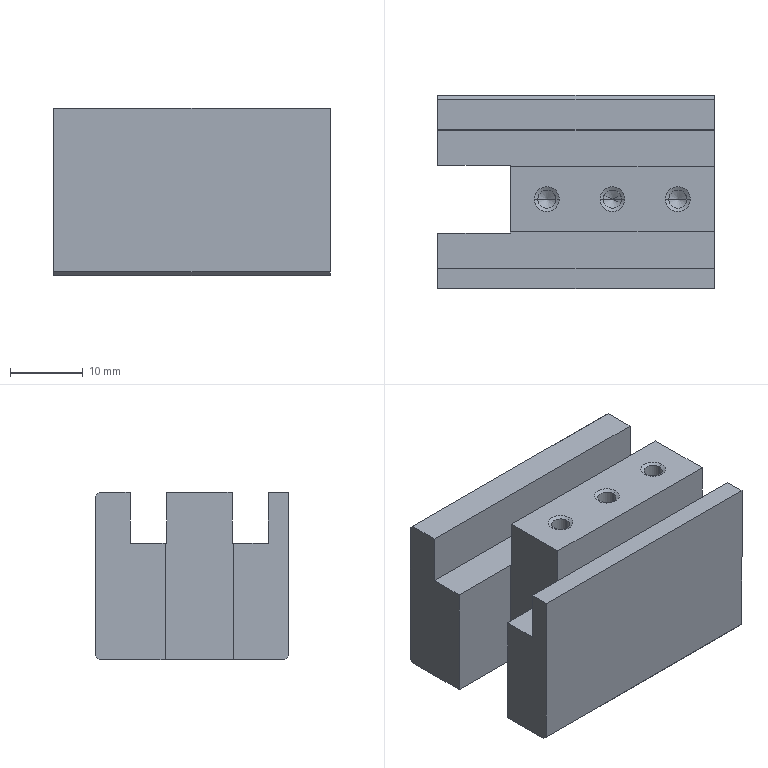Part | NX | 1 solid | 57 faces | box 38 x 26.5 x 22.95 mm | volume 17845 mm3 | cone 24 | plane 21 | cylinder 12 | commonest cylinder face diameters 2.5 x6 3.3 x6
STEP:
#1=CARTESIAN_POINT('',(0.,0.,-22.45));
#2=VERTEX_POINT('',#1);
#3=CARTESIAN_POINT('',(38.,0.,-22.45));
#4=VERTEX_POINT('',#3);
#5=CARTESIAN_POINT('',(0.,0.,-22.45));
#6=DIRECTION('',(1.,0.,0.));
#7=VECTOR('',#6,1000.);
#8=LINE('',#5,#7);
#9=EDGE_CURVE('',#2,#4,#8,.T.);
#10=ORIENTED_EDGE('',*,*,#9,.T.);
#11=CARTESIAN_POINT('',(38.,0.,0.));
#12=VERTEX_POINT('',#11);
#13=CARTESIAN_POINT('',(38.,0.,0.));
#14=DIRECTION('',(0.,0.,-1.));
#15=VECTOR('',#14,1000.);
#16=LINE('',#13,#15);
#17=EDGE_CURVE('',#12,#4,#16,.T.);
#18=ORIENTED_EDGE('',*,*,#17,.F.);
#19=CARTESIAN_POINT('',(0.,0.,0.));
#20=VERTEX_POINT('',#19);
#21=CARTESIAN_POINT('',(0.,0.,0.));
#22=DIRECTION('',(1.,0.,0.));
#23=VECTOR('',#22,1000.);
#24=LINE('',#21,#23);
#25=EDGE_CURVE('',#20,#12,#24,.T.);
#26=ORIENTED_EDGE('',*,*,#25,.F.);
#27=CARTESIAN_POINT('',(0.,0.,0.));
#28=DIRECTION('',(0.,0.,1.));
#29=VECTOR('',#28,1000.);
#30=LINE('',#27,#29);
#31=EDGE_CURVE('',#2,#20,#30,.T.);
#32=ORIENTED_EDGE('',*,*,#31,.F.);
#33=EDGE_LOOP('',(#10,#18,#26,#32));
#34=FACE_BOUND('',#33,.T.);
#35=CARTESIAN_POINT('',(0.,0.,0.));
#36=DIRECTION('',(0.,1.,0.));
#37=DIRECTION('',(1.,0.,0.));
#38=AXIS2_PLACEMENT_3D('',#35,#36,#37);
#39=PLANE('',#38);
#40=ADVANCED_FACE('',(#34),#39,.F.);
#41=CARTESIAN_POINT('',(0.,2.75,0.));
#42=VERTEX_POINT('',#41);
#43=CARTESIAN_POINT('',(38.,2.75,0.));
#44=VERTEX_POINT('',#43);
#45=CARTESIAN_POINT('',(0.,2.75,0.));
#46=DIRECTION('',(1.,0.,0.));
#47=VECTOR('',#46,1000.);
#48=LINE('',#45,#47);
#49=EDGE_CURVE('',#42,#44,#48,.T.);
#50=ORIENTED_EDGE('',*,*,#49,.F.);
#51=CARTESIAN_POINT('',(0.,0.,0.));
#52=DIRECTION('',(0.,1.,0.));
#53=VECTOR('',#52,1000.);
#54=LINE('',#51,#53);
#55=EDGE_CURVE('',#20,#42,#54,.T.);
#56=ORIENTED_EDGE('',*,*,#55,.F.);
#57=ORIENTED_EDGE('',*,*,#25,.T.);
#58=CARTESIAN_POINT('',(38.,0.,0.));
#59=DIRECTION('',(0.,-1.,0.));
#60=VECTOR('',#59,1000.);
#61=LINE('',#58,#60);
#62=EDGE_CURVE('',#44,#12,#61,.T.);
#63=ORIENTED_EDGE('',*,*,#62,.F.);
#64=EDGE_LOOP('',(#50,#56,#57,#63));
#65=FACE_BOUND('',#64,.T.);
#66=CARTESIAN_POINT('',(0.,0.,0.));
#67=DIRECTION('',(0.,0.,1.));
#68=DIRECTION('',(1.,0.,0.));
#69=AXIS2_PLACEMENT_3D('',#66,#67,#68);
#70=PLANE('',#69);
#71=ADVANCED_FACE('',(#65),#70,.T.);
#72=ORIENTED_EDGE('',*,*,#49,.T.);
#73=CARTESIAN_POINT('',(38.,2.75,-7.));
#74=VERTEX_POINT('',#73);
#75=CARTESIAN_POINT('',(38.,2.75,0.));
#76=DIRECTION('',(0.,0.,-1.));
#77=VECTOR('',#76,1000.);
#78=LINE('',#75,#77);
#79=EDGE_CURVE('',#44,#74,#78,.T.);
#80=ORIENTED_EDGE('',*,*,#79,.T.);
#81=CARTESIAN_POINT('',(0.,2.75,-7.));
#82=VERTEX_POINT('',#81);
#83=CARTESIAN_POINT('',(0.,2.75,-7.));
#84=DIRECTION('',(1.,0.,0.));
#85=VECTOR('',#84,1000.);
#86=LINE('',#83,#85);
#87=EDGE_CURVE('',#82,#74,#86,.T.);
#88=ORIENTED_EDGE('',*,*,#87,.F.);
#89=CARTESIAN_POINT('',(0.,2.75,0.));
#90=DIRECTION('',(0.,0.,1.));
#91=VECTOR('',#90,1000.);
#92=LINE('',#89,#91);
#93=EDGE_CURVE('',#82,#42,#92,.T.);
#94=ORIENTED_EDGE('',*,*,#93,.T.);
#95=EDGE_LOOP('',(#72,#80,#88,#94));
#96=FACE_BOUND('',#95,.T.);
#97=CARTESIAN_POINT('',(0.,2.75,-7.));
#98=DIRECTION('',(0.,-1.,0.));
#99=DIRECTION('',(0.,0.,-1.));
#100=AXIS2_PLACEMENT_3D('',#97,#98,#99);
#101=PLANE('',#100);
#102=ADVANCED_FACE('',(#96),#101,.F.);
#103=CARTESIAN_POINT('',(0.,7.55,-7.));
#104=VERTEX_POINT('',#103);
#105=CARTESIAN_POINT('',(0.,7.55,-22.95));
#106=VERTEX_POINT('',#105);
#107=CARTESIAN_POINT('',(0.,7.55,0.));
#108=DIRECTION('',(0.,0.,-1.));
#109=VECTOR('',#108,1000.);
#110=LINE('',#107,#109);
#111=EDGE_CURVE('',#104,#106,#110,.T.);
#112=ORIENTED_EDGE('',*,*,#111,.T.);
#113=CARTESIAN_POINT('',(0.,0.5,-22.95));
#114=VERTEX_POINT('',#113);
#115=CARTESIAN_POINT('',(0.,0.,-22.95));
#116=DIRECTION('',(0.,1.,0.));
#117=VECTOR('',#116,1000.);
#118=LINE('',#115,#117);
#119=EDGE_CURVE('',#114,#106,#118,.T.);
#120=ORIENTED_EDGE('',*,*,#119,.F.);
#121=CARTESIAN_POINT('',(0.,-22.45,0.));
#122=DIRECTION('',(0.,-0.7071,0.7071));
#123=VECTOR('',#122,1000.);
#124=LINE('',#121,#123);
#125=EDGE_CURVE('',#114,#2,#124,.T.);
#126=ORIENTED_EDGE('',*,*,#125,.T.);
#127=ORIENTED_EDGE('',*,*,#31,.T.);
#128=ORIENTED_EDGE('',*,*,#55,.T.);
#129=ORIENTED_EDGE('',*,*,#93,.F.);
#130=CARTESIAN_POINT('',(0.,0.,-7.));
#131=DIRECTION('',(0.,-1.,0.));
#132=VECTOR('',#131,1000.);
#133=LINE('',#130,#132);
#134=EDGE_CURVE('',#104,#82,#133,.T.);
#135=ORIENTED_EDGE('',*,*,#134,.F.);
#136=EDGE_LOOP('',(#112,#120,#126,#127,#128,#129,#135));
#137=FACE_BOUND('',#136,.T.);
#138=CARTESIAN_POINT('',(0.,0.,-23.));
#139=DIRECTION('',(-1.,0.,0.));
#140=DIRECTION('',(0.,0.,1.));
#141=AXIS2_PLACEMENT_3D('',#138,#139,#140);
#142=PLANE('',#141);
#143=ADVANCED_FACE('',(#137),#142,.T.);
#144=CARTESIAN_POINT('',(10.,7.55,-22.95));
#145=VERTEX_POINT('',#144);
#146=CARTESIAN_POINT('',(0.,7.55,-22.95));
#147=DIRECTION('',(1.,0.,0.));
#148=VECTOR('',#147,1000.);
#149=LINE('',#146,#148);
#150=EDGE_CURVE('',#106,#145,#149,.T.);
#151=ORIENTED_EDGE('',*,*,#150,.F.);
#152=ORIENTED_EDGE('',*,*,#111,.F.);
#153=CARTESIAN_POINT('',(10.,7.55,-7.));
#154=VERTEX_POINT('',#153);
#155=CARTESIAN_POINT('',(0.,7.55,-7.));
#156=DIRECTION('',(1.,0.,0.));
#157=VECTOR('',#156,1000.);
#158=LINE('',#155,#157);
#159=EDGE_CURVE('',#104,#154,#158,.T.);
#160=ORIENTED_EDGE('',*,*,#159,.T.);
#161=CARTESIAN_POINT('',(10.,7.55,0.));
#162=DIRECTION('',(0.,0.,1.));
#163=VECTOR('',#162,1000.);
#164=LINE('',#161,#163);
#165=EDGE_CURVE('',#145,#154,#164,.T.);
#166=ORIENTED_EDGE('',*,*,#165,.F.);
#167=EDGE_LOOP('',(#151,#152,#160,#166));
#168=FACE_BOUND('',#167,.T.);
#169=CARTESIAN_POINT('',(10.,7.55,-23.));
#170=DIRECTION('',(0.,-1.,0.));
#171=DIRECTION('',(0.,0.,-1.));
#172=AXIS2_PLACEMENT_3D('',#169,#170,#171);
#173=PLANE('',#172);
#174=ADVANCED_FACE('',(#168),#173,.F.);
#175=CARTESIAN_POINT('',(17.35,21.75,-10.8));
#176=VERTEX_POINT('',#175);
#177=CARTESIAN_POINT('',(20.65,21.75,-10.8));
#178=VERTEX_POINT('',#177);
#179=CARTESIAN_POINT('',(19.,21.75,-10.8));
#180=DIRECTION('',(0.,0.,-1.));
#181=DIRECTION('',(-1.,0.,0.));
#182=AXIS2_PLACEMENT_3D('',#179,#180,#181);
#183=CIRCLE('',#182,1.65);
#184=EDGE_CURVE('',#176,#178,#183,.T.);
#185=ORIENTED_EDGE('',*,*,#184,.T.);
#186=CARTESIAN_POINT('',(19.,21.75,-9.809));
#187=VERTEX_POINT('',#186);
#188=CARTESIAN_POINT('',(20.65,21.75,-10.8));
#189=DIRECTION('',(0.8572,0.,-0.515));
#190=VECTOR('',#189,1000.);
#191=LINE('',#188,#190);
#192=EDGE_CURVE('',#187,#178,#191,.T.);
#193=ORIENTED_EDGE('',*,*,#192,.F.);
#194=CARTESIAN_POINT('',(17.35,21.75,-10.8));
#195=DIRECTION('',(-0.8572,0.,-0.515));
#196=VECTOR('',#195,1000.);
#197=LINE('',#194,#196);
#198=EDGE_CURVE('',#187,#176,#197,.T.);
#199=ORIENTED_EDGE('',*,*,#198,.T.);
#200=EDGE_LOOP('',(#185,#193,#199));
#201=FACE_BOUND('',#200,.T.);
#202=CARTESIAN_POINT('',(19.,21.75,-10.8));
#203=DIRECTION('',(0.,0.,-1.));
#204=DIRECTION('',(-1.,0.,0.));
#205=AXIS2_PLACEMENT_3D('',#202,#203,#204);
#206=CONICAL_SURFACE('',#205,1.65,1.03);
#207=ADVANCED_FACE('',(#201),#206,.F.);
#208=CARTESIAN_POINT('',(10.,16.95,-22.95));
#209=VERTEX_POINT('',#208);
#210=CARTESIAN_POINT('',(0.,16.95,-22.95));
#211=VERTEX_POINT('',#210);
#212=CARTESIAN_POINT('',(0.,16.95,-22.95));
#213=DIRECTION('',(-1.,0.,0.));
#214=VECTOR('',#213,1000.);
#215=LINE('',#212,#214);
#216=EDGE_CURVE('',#209,#211,#215,.T.);
#217=ORIENTED_EDGE('',*,*,#216,.F.);
#218=CARTESIAN_POINT('',(10.,16.95,-7.));
#219=VERTEX_POINT('',#218);
#220=CARTESIAN_POINT('',(10.,16.95,0.));
#221=DIRECTION('',(0.,0.,1.));
#222=VECTOR('',#221,1000.);
#223=LINE('',#220,#222);
#224=EDGE_CURVE('',#209,#219,#223,.T.);
#225=ORIENTED_EDGE('',*,*,#224,.T.);
#226=CARTESIAN_POINT('',(0.,16.95,-7.));
#227=VERTEX_POINT('',#226);
#228=CARTESIAN_POINT('',(0.,16.95,-7.));
#229=DIRECTION('',(-1.,0.,0.));
#230=VECTOR('',#229,1000.);
#231=LINE('',#228,#230);
#232=EDGE_CURVE('',#219,#227,#231,.T.);
#233=ORIENTED_EDGE('',*,*,#232,.T.);
#234=CARTESIAN_POINT('',(0.,16.95,0.));
#235=DIRECTION('',(0.,0.,1.));
#236=VECTOR('',#235,1000.);
#237=LINE('',#234,#236);
#238=EDGE_CURVE('',#211,#227,#237,.T.);
#239=ORIENTED_EDGE('',*,*,#238,.F.);
#240=EDGE_LOOP('',(#217,#225,#233,#239));
#241=FACE_BOUND('',#240,.T.);
#242=CARTESIAN_POINT('',(0.,16.95,-23.));
#243=DIRECTION('',(0.,1.,0.));
#244=DIRECTION('',(1.,0.,0.));
#245=AXIS2_PLACEMENT_3D('',#242,#243,#244);
#246=PLANE('',#245);
#247=ADVANCED_FACE('',(#241),#246,.F.);
#248=ORIENTED_EDGE('',*,*,#238,.T.);
#249=CARTESIAN_POINT('',(0.,21.75,-7.));
#250=VERTEX_POINT('',#249);
#251=CARTESIAN_POINT('',(0.,0.,-7.));
#252=DIRECTION('',(0.,-1.,0.));
#253=VECTOR('',#252,1000.);
#254=LINE('',#251,#253);
#255=EDGE_CURVE('',#250,#227,#254,.T.);
#256=ORIENTED_EDGE('',*,*,#255,.F.);
#257=CARTESIAN_POINT('',(0.,21.75,0.));
#258=VERTEX_POINT('',#257);
#259=CARTESIAN_POINT('',(0.,21.75,0.));
#260=DIRECTION('',(0.,0.,-1.));
#261=VECTOR('',#260,1000.);
#262=LINE('',#259,#261);
#263=EDGE_CURVE('',#258,#250,#262,.T.);
#264=ORIENTED_EDGE('',*,*,#263,.F.);
#265=CARTESIAN_POINT('',(0.,26.,0.));
#266=VERTEX_POINT('',#265);
#267=CARTESIAN_POINT('',(0.,0.,0.));
#268=DIRECTION('',(0.,1.,0.));
#269=VECTOR('',#268,1000.);
#270=LINE('',#267,#269);
#271=EDGE_CURVE('',#258,#266,#270,.T.);
#272=ORIENTED_EDGE('',*,*,#271,.T.);
#273=CARTESIAN_POINT('',(0.,26.5,-0.5));
#274=VERTEX_POINT('',#273);
#275=CARTESIAN_POINT('',(0.,26.,0.));
#276=DIRECTION('',(0.,0.7071,-0.7071));
#277=VECTOR('',#276,1000.);
#278=LINE('',#275,#277);
#279=EDGE_CURVE('',#266,#274,#278,.T.);
#280=ORIENTED_EDGE('',*,*,#279,.T.);
#281=CARTESIAN_POINT('',(0.,26.5,-22.45));
#282=VERTEX_POINT('',#281);
#283=CARTESIAN_POINT('',(0.,26.5,0.));
#284=DIRECTION('',(0.,0.,1.));
#285=VECTOR('',#284,1000.);
#286=LINE('',#283,#285);
#287=EDGE_CURVE('',#282,#274,#286,.T.);
#288=ORIENTED_EDGE('',*,*,#287,.F.);
#289=CARTESIAN_POINT('',(0.,26.,-22.95));
#290=VERTEX_POINT('',#289);
#291=CARTESIAN_POINT('',(0.,48.95,0.));
#292=DIRECTION('',(0.,-0.7071,-0.7071));
#293=VECTOR('',#292,1000.);
#294=LINE('',#291,#293);
#295=EDGE_CURVE('',#282,#290,#294,.T.);
#296=ORIENTED_EDGE('',*,*,#295,.T.);
#297=CARTESIAN_POINT('',(0.,0.,-22.95));
#298=DIRECTION('',(0.,1.,0.));
#299=VECTOR('',#298,1000.);
#300=LINE('',#297,#299);
#301=EDGE_CURVE('',#211,#290,#300,.T.);
#302=ORIENTED_EDGE('',*,*,#301,.F.);
#303=EDGE_LOOP('',(#248,#256,#264,#272,#280,#288,#296,#302));
#304=FACE_BOUND('',#303,.T.);
#305=CARTESIAN_POINT('',(0.,0.,-23.));
#306=DIRECTION('',(-1.,0.,0.));
#307=DIRECTION('',(0.,0.,1.));
#308=AXIS2_PLACEMENT_3D('',#305,#306,#307);
#309=PLANE('',#308);
#310=ADVANCED_FACE('',(#304),#309,.T.);
#311=CARTESIAN_POINT('',(38.,26.5,-0.5));
#312=VERTEX_POINT('',#311);
#313=CARTESIAN_POINT('',(0.,26.5,-0.5));
#314=DIRECTION('',(1.,0.,0.));
#315=VECTOR('',#314,1000.);
#316=LINE('',#313,#315);
#317=EDGE_CURVE('',#274,#312,#316,.T.);
#318=ORIENTED_EDGE('',*,*,#317,.T.);
#319=CARTESIAN_POINT('',(38.,26.5,-22.45));
#320=VERTEX_POINT('',#319);
#321=CARTESIAN_POINT('',(38.,26.5,0.));
#322=DIRECTION('',(0.,0.,-1.));
#323=VECTOR('',#322,1000.);
#324=LINE('',#321,#323);
#325=EDGE_CURVE('',#312,#320,#324,.T.);
#326=ORIENTED_EDGE('',*,*,#325,.T.);
#327=CARTESIAN_POINT('',(0.,26.5,-22.45));
#328=DIRECTION('',(-1.,0.,0.));
#329=VECTOR('',#328,1000.);
#330=LINE('',#327,#329);
#331=EDGE_CURVE('',#320,#282,#330,.T.);
#332=ORIENTED_EDGE('',*,*,#331,.T.);
#333=ORIENTED_EDGE('',*,*,#287,.T.);
#334=EDGE_LOOP('',(#318,#326,#332,#333));
#335=FACE_BOUND('',#334,.T.);
#336=CARTESIAN_POINT('',(0.,26.5,0.));
#337=DIRECTION('',(0.,1.,0.));
#338=DIRECTION('',(1.,0.,0.));
#339=AXIS2_PLACEMENT_3D('',#336,#337,#338);
#340=PLANE('',#339);
#341=ADVANCED_FACE('',(#335),#340,.T.);
#342=CARTESIAN_POINT('',(38.,21.75,0.));
#343=VERTEX_POINT('',#342);
#344=CARTESIAN_POINT('',(0.,21.75,0.));
#345=DIRECTION('',(-1.,0.,0.));
#346=VECTOR('',#345,1000.);
#347=LINE('',#344,#346);
#348=EDGE_CURVE('',#343,#258,#347,.T.);
#349=ORIENTED_EDGE('',*,*,#348,.F.);
#350=CARTESIAN_POINT('',(38.,26.,0.));
#351=VERTEX_POINT('',#350);
#352=CARTESIAN_POINT('',(38.,0.,0.));
#353=DIRECTION('',(0.,1.,0.));
#354=VECTOR('',#353,1000.);
#355=LINE('',#352,#354);
#356=EDGE_CURVE('',#343,#351,#355,.T.);
#357=ORIENTED_EDGE('',*,*,#356,.T.);
#358=CARTESIAN_POINT('',(0.,26.,0.));
#359=DIRECTION('',(-1.,0.,0.));
#360=VECTOR('',#359,1000.);
#361=LINE('',#358,#360);
#362=EDGE_CURVE('',#351,#266,#361,.T.);
#363=ORIENTED_EDGE('',*,*,#362,.T.);
#364=ORIENTED_EDGE('',*,*,#271,.F.);
#365=EDGE_LOOP('',(#349,#357,#363,#364));
#366=FACE_BOUND('',#365,.T.);
#367=CARTESIAN_POINT('',(0.,0.,0.));
#368=DIRECTION('',(0.,0.,1.));
#369=DIRECTION('',(1.,0.,0.));
#370=AXIS2_PLACEMENT_3D('',#367,#368,#369);
#371=PLANE('',#370);
#372=ADVANCED_FACE('',(#366),#371,.T.);
#373=ORIENTED_EDGE('',*,*,#348,.T.);
#374=ORIENTED_EDGE('',*,*,#263,.T.);
#375=CARTESIAN_POINT('',(38.,21.75,-7.));
#376=VERTEX_POINT('',#375);
#377=CARTESIAN_POINT('',(0.,21.75,-7.));
#378=DIRECTION('',(1.,0.,0.));
#379=VECTOR('',#378,1000.);
#380=LINE('',#377,#379);
#381=EDGE_CURVE('',#250,#376,#380,.T.);
#382=ORIENTED_EDGE('',*,*,#381,.T.);
#383=CARTESIAN_POINT('',(38.,21.75,0.));
#384=DIRECTION('',(0.,0.,-1.));
#385=VECTOR('',#384,1000.);
#386=LINE('',#383,#385);
#387=EDGE_CURVE('',#343,#376,#386,.T.);
#388=ORIENTED_EDGE('',*,*,#387,.F.);
#389=EDGE_LOOP('',(#373,#374,#382,#388));
#390=FACE_BOUND('',#389,.T.);
#391=CARTESIAN_POINT('',(0.,21.75,0.));
#392=DIRECTION('',(0.,1.,0.));
#393=DIRECTION('',(1.,0.,0.));
#394=AXIS2_PLACEMENT_3D('',#391,#392,#393);
#395=PLANE('',#394);
#396=ADVANCED_FACE('',(#390),#395,.F.);
#397=ORIENTED_EDGE('',*,*,#387,.T.);
#398=CARTESIAN_POINT('',(38.,16.75,-7.));
#399=VERTEX_POINT('',#398);
#400=CARTESIAN_POINT('',(38.,0.,-7.));
#401=DIRECTION('',(0.,-1.,0.));
#402=VECTOR('',#401,1000.);
#403=LINE('',#400,#402);
#404=EDGE_CURVE('',#376,#399,#403,.T.);
#405=ORIENTED_EDGE('',*,*,#404,.T.);
#406=CARTESIAN_POINT('',(38.,16.75,0.));
#407=VERTEX_POINT('',#406);
#408=CARTESIAN_POINT('',(38.,16.75,0.));
#409=DIRECTION('',(0.,0.,1.));
#410=VECTOR('',#409,1000.);
#411=LINE('',#408,#410);
#412=EDGE_CURVE('',#399,#407,#411,.T.);
#413=ORIENTED_EDGE('',*,*,#412,.T.);
#414=CARTESIAN_POINT('',(38.,7.75,0.));
#415=VERTEX_POINT('',#414);
#416=CARTESIAN_POINT('',(38.,0.,0.));
#417=DIRECTION('',(0.,1.,0.));
#418=VECTOR('',#417,1000.);
#419=LINE('',#416,#418);
#420=EDGE_CURVE('',#415,#407,#419,.T.);
#421=ORIENTED_EDGE('',*,*,#420,.F.);
#422=CARTESIAN_POINT('',(38.,7.75,-7.));
#423=VERTEX_POINT('',#422);
#424=CARTESIAN_POINT('',(38.,7.75,0.));
#425=DIRECTION('',(0.,0.,-1.));
#426=VECTOR('',#425,1000.);
#427=LINE('',#424,#426);
#428=EDGE_CURVE('',#415,#423,#427,.T.);
#429=ORIENTED_EDGE('',*,*,#428,.T.);
#430=CARTESIAN_POINT('',(38.,0.,-7.));
#431=DIRECTION('',(0.,1.,0.));
#432=VECTOR('',#431,1000.);
#433=LINE('',#430,#432);
#434=EDGE_CURVE('',#74,#423,#433,.T.);
#435=ORIENTED_EDGE('',*,*,#434,.F.);
#436=ORIENTED_EDGE('',*,*,#79,.F.);
#437=ORIENTED_EDGE('',*,*,#62,.T.);
#438=ORIENTED_EDGE('',*,*,#17,.T.);
#439=CARTESIAN_POINT('',(38.,0.5,-22.95));
#440=VERTEX_POINT('',#439);
#441=CARTESIAN_POINT('',(38.,-22.45,0.));
#442=DIRECTION('',(0.,0.7071,-0.7071));
#443=VECTOR('',#442,1000.);
#444=LINE('',#441,#443);
#445=EDGE_CURVE('',#4,#440,#444,.T.);
#446=ORIENTED_EDGE('',*,*,#445,.T.);
#447=CARTESIAN_POINT('',(38.,26.,-22.95));
#448=VERTEX_POINT('',#447);
#449=CARTESIAN_POINT('',(38.,0.,-22.95));
#450=DIRECTION('',(0.,-1.,0.));
#451=VECTOR('',#450,1000.);
#452=LINE('',#449,#451);
#453=EDGE_CURVE('',#448,#440,#452,.T.);
#454=ORIENTED_EDGE('',*,*,#453,.F.);
#455=CARTESIAN_POINT('',(38.,48.95,0.));
#456=DIRECTION('',(0.,0.7071,0.7071));
#457=VECTOR('',#456,1000.);
#458=LINE('',#455,#457);
#459=EDGE_CURVE('',#448,#320,#458,.T.);
#460=ORIENTED_EDGE('',*,*,#459,.T.);
#461=ORIENTED_EDGE('',*,*,#325,.F.);
#462=CARTESIAN_POINT('',(38.,26.,0.));
#463=DIRECTION('',(0.,-0.7071,0.7071));
#464=VECTOR('',#463,1000.);
#465=LINE('',#462,#464);
#466=EDGE_CURVE('',#312,#351,#465,.T.);
#467=ORIENTED_EDGE('',*,*,#466,.T.);
#468=ORIENTED_EDGE('',*,*,#356,.F.);
#469=EDGE_LOOP('',(#397,#405,#413,#421,#429,#435,#436,#437,#438,#446,#454,#460,#461,#467,#468));
#470=FACE_BOUND('',#469,.T.);
#471=CARTESIAN_POINT('',(38.,0.,0.));
#472=DIRECTION('',(1.,0.,0.));
#473=DIRECTION('',(0.,1.,0.));
#474=AXIS2_PLACEMENT_3D('',#471,#472,#473);
#475=PLANE('',#474);
#476=ADVANCED_FACE('',(#470),#475,.T.);
#477=CARTESIAN_POINT('',(10.,7.75,-7.));
#478=VERTEX_POINT('',#477);
#479=CARTESIAN_POINT('',(10.,0.,-7.));
#480=DIRECTION('',(0.,1.,0.));
#481=VECTOR('',#480,1000.);
#482=LINE('',#479,#481);
#483=EDGE_CURVE('',#154,#478,#482,.T.);
#484=ORIENTED_EDGE('',*,*,#483,.F.);
#485=ORIENTED_EDGE('',*,*,#159,.F.);
#486=ORIENTED_EDGE('',*,*,#134,.T.);
#487=ORIENTED_EDGE('',*,*,#87,.T.);
#488=ORIENTED_EDGE('',*,*,#434,.T.);
#489=CARTESIAN_POINT('',(0.,7.75,-7.));
#490=DIRECTION('',(-1.,0.,0.));
#491=VECTOR('',#490,1000.);
#492=LINE('',#489,#491);
#493=EDGE_CURVE('',#423,#478,#492,.T.);
#494=ORIENTED_EDGE('',*,*,#493,.T.);
#495=EDGE_LOOP('',(#484,#485,#486,#487,#488,#494));
#496=FACE_BOUND('',#495,.T.);
#497=CARTESIAN_POINT('',(0.,9.25,-7.));
#498=DIRECTION('',(0.,0.,-1.));
#499=DIRECTION('',(0.,-1.,0.));
#500=AXIS2_PLACEMENT_3D('',#497,#498,#499);
#501=PLANE('',#500);
#502=ADVANCED_FACE('',(#496),#501,.F.);
#503=CARTESIAN_POINT('',(10.,16.75,0.));
#504=VERTEX_POINT('',#503);
#505=CARTESIAN_POINT('',(10.,7.75,0.));
#506=VERTEX_POINT('',#505);
#507=CARTESIAN_POINT('',(10.,0.,0.));
#508=DIRECTION('',(0.,-1.,0.));
#509=VECTOR('',#508,1000.);
#510=LINE('',#507,#509);
#511=EDGE_CURVE('',#504,#506,#510,.T.);
#512=ORIENTED_EDGE('',*,*,#511,.F.);
#513=CARTESIAN_POINT('',(10.,16.75,-7.));
#514=VERTEX_POINT('',#513);
#515=CARTESIAN_POINT('',(10.,16.75,0.));
#516=DIRECTION('',(0.,0.,1.));
#517=VECTOR('',#516,1000.);
#518=LINE('',#515,#517);
#519=EDGE_CURVE('',#514,#504,#518,.T.);
#520=ORIENTED_EDGE('',*,*,#519,.F.);
#521=CARTESIAN_POINT('',(10.,0.,-7.));
#522=DIRECTION('',(0.,1.,0.));
#523=VECTOR('',#522,1000.);
#524=LINE('',#521,#523);
#525=EDGE_CURVE('',#514,#219,#524,.T.);
#526=ORIENTED_EDGE('',*,*,#525,.T.);
#527=ORIENTED_EDGE('',*,*,#224,.F.);
#528=CARTESIAN_POINT('',(10.,0.,-22.95));
#529=DIRECTION('',(0.,1.,0.));
#530=VECTOR('',#529,1000.);
#531=LINE('',#528,#530);
#532=EDGE_CURVE('',#145,#209,#531,.T.);
#533=ORIENTED_EDGE('',*,*,#532,.F.);
#534=ORIENTED_EDGE('',*,*,#165,.T.);
#535=ORIENTED_EDGE('',*,*,#483,.T.);
#536=CARTESIAN_POINT('',(10.,7.75,0.));
#537=DIRECTION('',(0.,0.,-1.));
#538=VECTOR('',#537,1000.);
#539=LINE('',#536,#538);
#540=EDGE_CURVE('',#506,#478,#539,.T.);
#541=ORIENTED_EDGE('',*,*,#540,.F.);
#542=EDGE_LOOP('',(#512,#520,#526,#527,#533,#534,#535,#541));
#543=FACE_BOUND('',#542,.T.);
#544=CARTESIAN_POINT('',(10.,16.95,-23.));
#545=DIRECTION('',(1.,0.,0.));
#546=DIRECTION('',(0.,1.,0.));
#547=AXIS2_PLACEMENT_3D('',#544,#545,#546);
#548=PLANE('',#547);
#549=ADVANCED_FACE('',(#543),#548,.F.);
#550=CARTESIAN_POINT('',(0.,7.75,0.));
#551=DIRECTION('',(1.,0.,0.));
#552=VECTOR('',#551,1000.);
#553=LINE('',#550,#552);
#554=EDGE_CURVE('',#506,#415,#553,.T.);
#555=ORIENTED_EDGE('',*,*,#554,.T.);
#556=ORIENTED_EDGE('',*,*,#420,.T.);
#557=CARTESIAN_POINT('',(0.,16.75,0.));
#558=DIRECTION('',(-1.,0.,0.));
#559=VECTOR('',#558,1000.);
#560=LINE('',#557,#559);
#561=EDGE_CURVE('',#407,#504,#560,.T.);
#562=ORIENTED_EDGE('',*,*,#561,.T.);
#563=ORIENTED_EDGE('',*,*,#511,.T.);
#564=EDGE_LOOP('',(#555,#556,#562,#563));
#565=FACE_BOUND('',#564,.T.);
#566=CARTESIAN_POINT('',(31.3,12.25,0.));
#567=VERTEX_POINT('',#566);
#568=CARTESIAN_POINT('',(34.7,12.25,0.));
#569=VERTEX_POINT('',#568);
#570=CARTESIAN_POINT('',(33.,12.25,0.));
#571=DIRECTION('',(0.,0.,1.));
#572=DIRECTION('',(1.,0.,0.));
#573=AXIS2_PLACEMENT_3D('',#570,#571,#572);
#574=CIRCLE('',#573,1.7);
#575=EDGE_CURVE('',#567,#569,#574,.T.);
#576=ORIENTED_EDGE('',*,*,#575,.F.);
#577=CARTESIAN_POINT('',(33.,12.25,0.));
#578=DIRECTION('',(0.,0.,1.));
#579=DIRECTION('',(1.,0.,0.));
#580=AXIS2_PLACEMENT_3D('',#577,#578,#579);
#581=CIRCLE('',#580,1.7);
#582=EDGE_CURVE('',#569,#567,#581,.T.);
#583=ORIENTED_EDGE('',*,*,#582,.F.);
#584=EDGE_LOOP('',(#576,#583));
#585=FACE_BOUND('',#584,.T.);
#586=CARTESIAN_POINT('',(22.3,12.25,0.));
#587=VERTEX_POINT('',#586);
#588=CARTESIAN_POINT('',(25.7,12.25,0.));
#589=VERTEX_POINT('',#588);
#590=CARTESIAN_POINT('',(24.,12.25,0.));
#591=DIRECTION('',(0.,0.,1.));
#592=DIRECTION('',(1.,0.,0.));
#593=AXIS2_PLACEMENT_3D('',#590,#591,#592);
#594=CIRCLE('',#593,1.7);
#595=EDGE_CURVE('',#587,#589,#594,.T.);
#596=ORIENTED_EDGE('',*,*,#595,.F.);
#597=CARTESIAN_POINT('',(24.,12.25,0.));
#598=DIRECTION('',(0.,0.,1.));
#599=DIRECTION('',(1.,0.,0.));
#600=AXIS2_PLACEMENT_3D('',#597,#598,#599);
#601=CIRCLE('',#600,1.7);
#602=EDGE_CURVE('',#589,#587,#601,.T.);
#603=ORIENTED_EDGE('',*,*,#602,.F.);
#604=EDGE_LOOP('',(#596,#603));
#605=FACE_BOUND('',#604,.T.);
#606=CARTESIAN_POINT('',(13.3,12.25,0.));
#607=VERTEX_POINT('',#606);
#608=CARTESIAN_POINT('',(16.7,12.25,0.));
#609=VERTEX_POINT('',#608);
#610=CARTESIAN_POINT('',(15.,12.25,0.));
#611=DIRECTION('',(0.,0.,1.));
#612=DIRECTION('',(1.,0.,0.));
#613=AXIS2_PLACEMENT_3D('',#610,#611,#612);
#614=CIRCLE('',#613,1.7);
#615=EDGE_CURVE('',#607,#609,#614,.T.);
#616=ORIENTED_EDGE('',*,*,#615,.F.);
#617=CARTESIAN_POINT('',(15.,12.25,0.));
#618=DIRECTION('',(0.,0.,1.));
#619=DIRECTION('',(1.,0.,0.));
#620=AXIS2_PLACEMENT_3D('',#617,#618,#619);
#621=CIRCLE('',#620,1.7);
#622=EDGE_CURVE('',#609,#607,#621,.T.);
#623=ORIENTED_EDGE('',*,*,#622,.F.);
#624=EDGE_LOOP('',(#616,#623));
#625=FACE_BOUND('',#624,.T.);
#626=CARTESIAN_POINT('',(0.,1.25,0.));
#627=DIRECTION('',(0.,0.,1.));
#628=DIRECTION('',(1.,0.,0.));
#629=AXIS2_PLACEMENT_3D('',#626,#627,#628);
#630=PLANE('',#629);
#631=ADVANCED_FACE('',(#565,#585,#605,#625),#630,.T.);
#632=ORIENTED_EDGE('',*,*,#519,.T.);
#633=ORIENTED_EDGE('',*,*,#561,.F.);
#634=ORIENTED_EDGE('',*,*,#412,.F.);
#635=CARTESIAN_POINT('',(0.,16.75,-7.));
#636=DIRECTION('',(1.,0.,0.));
#637=VECTOR('',#636,1000.);
#638=LINE('',#635,#637);
#639=EDGE_CURVE('',#514,#399,#638,.T.);
#640=ORIENTED_EDGE('',*,*,#639,.F.);
#641=EDGE_LOOP('',(#632,#633,#634,#640));
#642=FACE_BOUND('',#641,.T.);
#643=CARTESIAN_POINT('',(0.,16.75,-7.));
#644=DIRECTION('',(0.,-1.,0.));
#645=DIRECTION('',(0.,0.,-1.));
#646=AXIS2_PLACEMENT_3D('',#643,#644,#645);
#647=PLANE('',#646);
#648=ADVANCED_FACE('',(#642),#647,.F.);
#649=ORIENTED_EDGE('',*,*,#232,.F.);
#650=ORIENTED_EDGE('',*,*,#525,.F.);
#651=ORIENTED_EDGE('',*,*,#639,.T.);
#652=ORIENTED_EDGE('',*,*,#404,.F.);
#653=ORIENTED_EDGE('',*,*,#381,.F.);
#654=ORIENTED_EDGE('',*,*,#255,.T.);
#655=EDGE_LOOP('',(#649,#650,#651,#652,#653,#654));
#656=FACE_BOUND('',#655,.T.);
#657=CARTESIAN_POINT('',(0.,23.25,-7.));
#658=DIRECTION('',(0.,0.,-1.));
#659=DIRECTION('',(0.,-1.,0.));
#660=AXIS2_PLACEMENT_3D('',#657,#658,#659);
#661=PLANE('',#660);
#662=ADVANCED_FACE('',(#656),#661,.F.);
#663=ORIENTED_EDGE('',*,*,#540,.T.);
#664=ORIENTED_EDGE('',*,*,#493,.F.);
#665=ORIENTED_EDGE('',*,*,#428,.F.);
#666=ORIENTED_EDGE('',*,*,#554,.F.);
#667=EDGE_LOOP('',(#663,#664,#665,#666));
#668=FACE_BOUND('',#667,.T.);
#669=CARTESIAN_POINT('',(0.,7.75,0.));
#670=DIRECTION('',(0.,1.,0.));
#671=DIRECTION('',(1.,0.,0.));
#672=AXIS2_PLACEMENT_3D('',#669,#670,#671);
#673=PLANE('',#672);
#674=ADVANCED_FACE('',(#668),#673,.F.);
#675=ORIENTED_EDGE('',*,*,#184,.F.);
#676=CARTESIAN_POINT('',(17.35,21.75,-22.566));
#677=VERTEX_POINT('',#676);
#678=CARTESIAN_POINT('',(17.35,21.75,-23.));
#679=DIRECTION('',(0.,0.,-1.));
#680=VECTOR('',#679,1000.);
#681=LINE('',#678,#680);
#682=EDGE_CURVE('',#677,#176,#681,.F.);
#683=ORIENTED_EDGE('',*,*,#682,.F.);
#684=CARTESIAN_POINT('',(20.65,21.75,-22.566));
#685=VERTEX_POINT('',#684);
#686=CARTESIAN_POINT('',(19.,21.75,-22.566));
#687=DIRECTION('',(0.,0.,-1.));
#688=DIRECTION('',(-1.,0.,0.));
#689=AXIS2_PLACEMENT_3D('',#686,#687,#688);
#690=CIRCLE('',#689,1.65);
#691=EDGE_CURVE('',#677,#685,#690,.T.);
#692=ORIENTED_EDGE('',*,*,#691,.T.);
#693=CARTESIAN_POINT('',(20.65,21.75,-23.));
#694=DIRECTION('',(0.,0.,-1.));
#695=VECTOR('',#694,1000.);
#696=LINE('',#693,#695);
#697=EDGE_CURVE('',#685,#178,#696,.F.);
#698=ORIENTED_EDGE('',*,*,#697,.T.);
#699=EDGE_LOOP('',(#675,#683,#692,#698));
#700=FACE_BOUND('',#699,.T.);
#701=CARTESIAN_POINT('',(19.,21.75,-23.));
#702=DIRECTION('',(0.,0.,-1.));
#703=DIRECTION('',(-1.,0.,0.));
#704=AXIS2_PLACEMENT_3D('',#701,#702,#703);
#705=CYLINDRICAL_SURFACE('',#704,1.65);
#706=ADVANCED_FACE('',(#700),#705,.F.);
#707=CARTESIAN_POINT('',(16.685,21.75,-22.95));
#708=VERTEX_POINT('',#707);
#709=CARTESIAN_POINT('',(21.315,21.75,-22.95));
#710=VERTEX_POINT('',#709);
#711=CARTESIAN_POINT('',(19.,21.75,-22.95));
#712=DIRECTION('',(0.,0.,-1.));
#713=DIRECTION('',(-1.,0.,0.));
#714=AXIS2_PLACEMENT_3D('',#711,#712,#713);
#715=CIRCLE('',#714,2.315);
#716=EDGE_CURVE('',#708,#710,#715,.T.);
#717=ORIENTED_EDGE('',*,*,#716,.T.);
#718=CARTESIAN_POINT('',(20.65,21.75,-22.566));
#719=DIRECTION('',(0.866,0.,-0.5));
#720=VECTOR('',#719,1000.);
#721=LINE('',#718,#720);
#722=EDGE_CURVE('',#710,#685,#721,.F.);
#723=ORIENTED_EDGE('',*,*,#722,.T.);
#724=ORIENTED_EDGE('',*,*,#691,.F.);
#725=CARTESIAN_POINT('',(17.35,21.75,-22.566));
#726=DIRECTION('',(-0.866,0.,-0.5));
#727=VECTOR('',#726,1000.);
#728=LINE('',#725,#727);
#729=EDGE_CURVE('',#708,#677,#728,.F.);
#730=ORIENTED_EDGE('',*,*,#729,.F.);
#731=EDGE_LOOP('',(#717,#723,#724,#730));
#732=FACE_BOUND('',#731,.T.);
#733=CARTESIAN_POINT('',(19.,21.75,-22.566));
#734=DIRECTION('',(0.,0.,-1.));
#735=DIRECTION('',(-1.,0.,0.));
#736=AXIS2_PLACEMENT_3D('',#733,#734,#735);
#737=CONICAL_SURFACE('',#736,1.65,1.047);
#738=ADVANCED_FACE('',(#732),#737,.F.);
#739=CARTESIAN_POINT('',(0.,26.,-22.95));
#740=DIRECTION('',(1.,0.,0.));
#741=VECTOR('',#740,1000.);
#742=LINE('',#739,#741);
#743=EDGE_CURVE('',#290,#448,#742,.T.);
#744=ORIENTED_EDGE('',*,*,#743,.F.);
#745=ORIENTED_EDGE('',*,*,#295,.F.);
#746=ORIENTED_EDGE('',*,*,#331,.F.);
#747=ORIENTED_EDGE('',*,*,#459,.F.);
#748=EDGE_LOOP('',(#744,#745,#746,#747));
#749=FACE_BOUND('',#748,.T.);
#750=CARTESIAN_POINT('',(19.,26.25,-22.7));
#751=DIRECTION('',(0.,-0.7071,0.7071));
#752=DIRECTION('',(-1.,0.,0.));
#753=AXIS2_PLACEMENT_3D('',#750,#751,#752);
#754=PLANE('',#753);
#755=ADVANCED_FACE('',(#749),#754,.F.);
#756=ORIENTED_EDGE('',*,*,#743,.T.);
#757=ORIENTED_EDGE('',*,*,#453,.T.);
#758=CARTESIAN_POINT('',(0.,0.5,-22.95));
#759=DIRECTION('',(-1.,0.,0.));
#760=VECTOR('',#759,1000.);
#761=LINE('',#758,#760);
#762=EDGE_CURVE('',#440,#114,#761,.T.);
#763=ORIENTED_EDGE('',*,*,#762,.T.);
#764=ORIENTED_EDGE('',*,*,#119,.T.);
#765=ORIENTED_EDGE('',*,*,#150,.T.);
#766=ORIENTED_EDGE('',*,*,#532,.T.);
#767=ORIENTED_EDGE('',*,*,#216,.T.);
#768=ORIENTED_EDGE('',*,*,#301,.T.);
#769=EDGE_LOOP('',(#756,#757,#763,#764,#765,#766,#767,#768));
#770=FACE_BOUND('',#769,.T.);
#771=CARTESIAN_POINT('',(30.685,21.75,-22.95));
#772=VERTEX_POINT('',#771);
#773=CARTESIAN_POINT('',(35.315,21.75,-22.95));
#774=VERTEX_POINT('',#773);
#775=CARTESIAN_POINT('',(33.,21.75,-22.95));
#776=DIRECTION('',(0.,0.,-1.));
#777=DIRECTION('',(-1.,0.,0.));
#778=AXIS2_PLACEMENT_3D('',#775,#776,#777);
#779=CIRCLE('',#778,2.315);
#780=EDGE_CURVE('',#772,#774,#779,.T.);
#781=ORIENTED_EDGE('',*,*,#780,.F.);
#782=CARTESIAN_POINT('',(33.,21.75,-22.95));
#783=DIRECTION('',(0.,0.,-1.));
#784=DIRECTION('',(-1.,0.,0.));
#785=AXIS2_PLACEMENT_3D('',#782,#783,#784);
#786=CIRCLE('',#785,2.315);
#787=EDGE_CURVE('',#774,#772,#786,.T.);
#788=ORIENTED_EDGE('',*,*,#787,.F.);
#789=EDGE_LOOP('',(#781,#788));
#790=FACE_BOUND('',#789,.T.);
#791=CARTESIAN_POINT('',(7.315,21.75,-22.95));
#792=VERTEX_POINT('',#791);
#793=CARTESIAN_POINT('',(2.685,21.75,-22.95));
#794=VERTEX_POINT('',#793);
#795=CARTESIAN_POINT('',(5.,21.75,-22.95));
#796=DIRECTION('',(0.,0.,-1.));
#797=DIRECTION('',(-1.,0.,0.));
#798=AXIS2_PLACEMENT_3D('',#795,#796,#797);
#799=CIRCLE('',#798,2.315);
#800=EDGE_CURVE('',#792,#794,#799,.T.);
#801=ORIENTED_EDGE('',*,*,#800,.F.);
#802=CARTESIAN_POINT('',(5.,21.75,-22.95));
#803=DIRECTION('',(0.,0.,-1.));
#804=DIRECTION('',(-1.,0.,0.));
#805=AXIS2_PLACEMENT_3D('',#802,#803,#804);
#806=CIRCLE('',#805,2.315);
#807=EDGE_CURVE('',#794,#792,#806,.T.);
#808=ORIENTED_EDGE('',*,*,#807,.F.);
#809=EDGE_LOOP('',(#801,#808));
#810=FACE_BOUND('',#809,.T.);
#811=ORIENTED_EDGE('',*,*,#716,.F.);
#812=CARTESIAN_POINT('',(19.,21.75,-22.95));
#813=DIRECTION('',(0.,0.,-1.));
#814=DIRECTION('',(-1.,0.,0.));
#815=AXIS2_PLACEMENT_3D('',#812,#813,#814);
#816=CIRCLE('',#815,2.315);
#817=EDGE_CURVE('',#710,#708,#816,.T.);
#818=ORIENTED_EDGE('',*,*,#817,.F.);
#819=EDGE_LOOP('',(#811,#818));
#820=FACE_BOUND('',#819,.T.);
#821=CARTESIAN_POINT('',(38.,0.,-22.95));
#822=DIRECTION('',(0.,0.,-1.));
#823=DIRECTION('',(0.,-1.,0.));
#824=AXIS2_PLACEMENT_3D('',#821,#822,#823);
#825=PLANE('',#824);
#826=ADVANCED_FACE('',(#770,#790,#810,#820),#825,.T.);
#827=CARTESIAN_POINT('',(6.65,21.75,-10.8));
#828=VERTEX_POINT('',#827);
#829=CARTESIAN_POINT('',(3.35,21.75,-10.8));
#830=VERTEX_POINT('',#829);
#831=CARTESIAN_POINT('',(5.,21.75,-10.8));
#832=DIRECTION('',(0.,0.,-1.));
#833=DIRECTION('',(-1.,0.,0.));
#834=AXIS2_PLACEMENT_3D('',#831,#832,#833);
#835=CIRCLE('',#834,1.65);
#836=EDGE_CURVE('',#828,#830,#835,.T.);
#837=ORIENTED_EDGE('',*,*,#836,.F.);
#838=CARTESIAN_POINT('',(6.65,21.75,-22.566));
#839=VERTEX_POINT('',#838);
#840=CARTESIAN_POINT('',(6.65,21.75,-23.));
#841=DIRECTION('',(0.,0.,-1.));
#842=VECTOR('',#841,1000.);
#843=LINE('',#840,#842);
#844=EDGE_CURVE('',#828,#839,#843,.T.);
#845=ORIENTED_EDGE('',*,*,#844,.T.);
#846=CARTESIAN_POINT('',(3.35,21.75,-22.566));
#847=VERTEX_POINT('',#846);
#848=CARTESIAN_POINT('',(5.,21.75,-22.566));
#849=DIRECTION('',(0.,0.,-1.));
#850=DIRECTION('',(-1.,0.,0.));
#851=AXIS2_PLACEMENT_3D('',#848,#849,#850);
#852=CIRCLE('',#851,1.65);
#853=EDGE_CURVE('',#839,#847,#852,.T.);
#854=ORIENTED_EDGE('',*,*,#853,.T.);
#855=CARTESIAN_POINT('',(3.35,21.75,-23.));
#856=DIRECTION('',(0.,0.,-1.));
#857=VECTOR('',#856,1000.);
#858=LINE('',#855,#857);
#859=EDGE_CURVE('',#830,#847,#858,.T.);
#860=ORIENTED_EDGE('',*,*,#859,.F.);
#861=EDGE_LOOP('',(#837,#845,#854,#860));
#862=FACE_BOUND('',#861,.T.);
#863=CARTESIAN_POINT('',(5.,21.75,-23.));
#864=DIRECTION('',(0.,0.,-1.));
#865=DIRECTION('',(-1.,0.,0.));
#866=AXIS2_PLACEMENT_3D('',#863,#864,#865);
#867=CYLINDRICAL_SURFACE('',#866,1.65);
#868=ADVANCED_FACE('',(#862),#867,.F.);
#869=ORIENTED_EDGE('',*,*,#317,.F.);
#870=ORIENTED_EDGE('',*,*,#279,.F.);
#871=ORIENTED_EDGE('',*,*,#362,.F.);
#872=ORIENTED_EDGE('',*,*,#466,.F.);
#873=EDGE_LOOP('',(#869,#870,#871,#872));
#874=FACE_BOUND('',#873,.T.);
#875=CARTESIAN_POINT('',(19.,26.25,-0.25));
#876=DIRECTION('',(0.,-0.7071,-0.7071));
#877=DIRECTION('',(0.,-0.7071,0.7071));
#878=AXIS2_PLACEMENT_3D('',#875,#876,#877);
#879=PLANE('',#878);
#880=ADVANCED_FACE('',(#874),#879,.F.);
#881=ORIENTED_EDGE('',*,*,#836,.T.);
#882=CARTESIAN_POINT('',(5.,21.75,-9.809));
#883=VERTEX_POINT('',#882);
#884=CARTESIAN_POINT('',(3.35,21.75,-10.8));
#885=DIRECTION('',(-0.8572,0.,-0.515));
#886=VECTOR('',#885,1000.);
#887=LINE('',#884,#886);
#888=EDGE_CURVE('',#883,#830,#887,.T.);
#889=ORIENTED_EDGE('',*,*,#888,.F.);
#890=CARTESIAN_POINT('',(6.65,21.75,-10.8));
#891=DIRECTION('',(0.8572,0.,-0.515));
#892=VECTOR('',#891,1000.);
#893=LINE('',#890,#892);
#894=EDGE_CURVE('',#883,#828,#893,.T.);
#895=ORIENTED_EDGE('',*,*,#894,.T.);
#896=EDGE_LOOP('',(#881,#889,#895));
#897=FACE_BOUND('',#896,.T.);
#898=CARTESIAN_POINT('',(5.,21.75,-10.8));
#899=DIRECTION('',(0.,0.,-1.));
#900=DIRECTION('',(-1.,0.,0.));
#901=AXIS2_PLACEMENT_3D('',#898,#899,#900);
#902=CONICAL_SURFACE('',#901,1.65,1.03);
#903=ADVANCED_FACE('',(#897),#902,.F.);
#904=CARTESIAN_POINT('',(5.,21.75,-22.566));
#905=DIRECTION('',(0.,0.,-1.));
#906=DIRECTION('',(-1.,0.,0.));
#907=AXIS2_PLACEMENT_3D('',#904,#905,#906);
#908=CIRCLE('',#907,1.65);
#909=EDGE_CURVE('',#847,#839,#908,.T.);
#910=ORIENTED_EDGE('',*,*,#909,.F.);
#911=CARTESIAN_POINT('',(3.35,21.75,-22.566));
#912=DIRECTION('',(-0.866,0.,-0.5));
#913=VECTOR('',#912,1000.);
#914=LINE('',#911,#913);
#915=EDGE_CURVE('',#794,#847,#914,.F.);
#916=ORIENTED_EDGE('',*,*,#915,.F.);
#917=ORIENTED_EDGE('',*,*,#807,.T.);
#918=CARTESIAN_POINT('',(6.65,21.75,-22.566));
#919=DIRECTION('',(0.866,0.,-0.5));
#920=VECTOR('',#919,1000.);
#921=LINE('',#918,#920);
#922=EDGE_CURVE('',#792,#839,#921,.F.);
#923=ORIENTED_EDGE('',*,*,#922,.T.);
#924=EDGE_LOOP('',(#910,#916,#917,#923));
#925=FACE_BOUND('',#924,.T.);
#926=CARTESIAN_POINT('',(5.,21.75,-22.566));
#927=DIRECTION('',(0.,0.,-1.));
#928=DIRECTION('',(-1.,0.,0.));
#929=AXIS2_PLACEMENT_3D('',#926,#927,#928);
#930=CONICAL_SURFACE('',#929,1.65,1.047);
#931=ADVANCED_FACE('',(#925),#930,.F.);
#932=CARTESIAN_POINT('',(31.35,21.75,-22.566));
#933=VERTEX_POINT('',#932);
#934=CARTESIAN_POINT('',(34.65,21.75,-22.566));
#935=VERTEX_POINT('',#934);
#936=CARTESIAN_POINT('',(33.,21.75,-22.566));
#937=DIRECTION('',(0.,0.,-1.));
#938=DIRECTION('',(-1.,0.,0.));
#939=AXIS2_PLACEMENT_3D('',#936,#937,#938);
#940=CIRCLE('',#939,1.65);
#941=EDGE_CURVE('',#933,#935,#940,.T.);
#942=ORIENTED_EDGE('',*,*,#941,.T.);
#943=CARTESIAN_POINT('',(34.65,21.75,-10.8));
#944=VERTEX_POINT('',#943);
#945=CARTESIAN_POINT('',(34.65,21.75,-23.));
#946=DIRECTION('',(0.,0.,-1.));
#947=VECTOR('',#946,1000.);
#948=LINE('',#945,#947);
#949=EDGE_CURVE('',#944,#935,#948,.T.);
#950=ORIENTED_EDGE('',*,*,#949,.F.);
#951=CARTESIAN_POINT('',(31.35,21.75,-10.8));
#952=VERTEX_POINT('',#951);
#953=CARTESIAN_POINT('',(33.,21.75,-10.8));
#954=DIRECTION('',(0.,0.,-1.));
#955=DIRECTION('',(-1.,0.,0.));
#956=AXIS2_PLACEMENT_3D('',#953,#954,#955);
#957=CIRCLE('',#956,1.65);
#958=EDGE_CURVE('',#952,#944,#957,.T.);
#959=ORIENTED_EDGE('',*,*,#958,.F.);
#960=CARTESIAN_POINT('',(31.35,21.75,-23.));
#961=DIRECTION('',(0.,0.,-1.));
#962=VECTOR('',#961,1000.);
#963=LINE('',#960,#962);
#964=EDGE_CURVE('',#952,#933,#963,.T.);
#965=ORIENTED_EDGE('',*,*,#964,.T.);
#966=EDGE_LOOP('',(#942,#950,#959,#965));
#967=FACE_BOUND('',#966,.T.);
#968=CARTESIAN_POINT('',(33.,21.75,-23.));
#969=DIRECTION('',(0.,0.,-1.));
#970=DIRECTION('',(-1.,0.,0.));
#971=AXIS2_PLACEMENT_3D('',#968,#969,#970);
#972=CYLINDRICAL_SURFACE('',#971,1.65);
#973=ADVANCED_FACE('',(#967),#972,.F.);
#974=ORIENTED_EDGE('',*,*,#9,.F.);
#975=ORIENTED_EDGE('',*,*,#125,.F.);
#976=ORIENTED_EDGE('',*,*,#762,.F.);
#977=ORIENTED_EDGE('',*,*,#445,.F.);
#978=EDGE_LOOP('',(#974,#975,#976,#977));
#979=FACE_BOUND('',#978,.T.);
#980=CARTESIAN_POINT('',(19.,0.25,-22.7));
#981=DIRECTION('',(0.,0.7071,0.7071));
#982=DIRECTION('',(1.,0.,0.));
#983=AXIS2_PLACEMENT_3D('',#980,#981,#982);
#984=PLANE('',#983);
#985=ADVANCED_FACE('',(#979),#984,.F.);
#986=CARTESIAN_POINT('',(33.,21.75,-9.809));
#987=VERTEX_POINT('',#986);
#988=CARTESIAN_POINT('',(34.65,21.75,-10.8));
#989=DIRECTION('',(0.8572,0.,-0.515));
#990=VECTOR('',#989,1000.);
#991=LINE('',#988,#990);
#992=EDGE_CURVE('',#987,#944,#991,.T.);
#993=ORIENTED_EDGE('',*,*,#992,.T.);
#994=CARTESIAN_POINT('',(33.,21.75,-10.8));
#995=DIRECTION('',(0.,0.,-1.));
#996=DIRECTION('',(-1.,0.,0.));
#997=AXIS2_PLACEMENT_3D('',#994,#995,#996);
#998=CIRCLE('',#997,1.65);
#999=EDGE_CURVE('',#944,#952,#998,.T.);
#1000=ORIENTED_EDGE('',*,*,#999,.T.);
#1001=CARTESIAN_POINT('',(31.35,21.75,-10.8));
#1002=DIRECTION('',(-0.8572,0.,-0.515));
#1003=VECTOR('',#1002,1000.);
#1004=LINE('',#1001,#1003);
#1005=EDGE_CURVE('',#987,#952,#1004,.T.);
#1006=ORIENTED_EDGE('',*,*,#1005,.F.);
#1007=EDGE_LOOP('',(#993,#1000,#1006));
#1008=FACE_BOUND('',#1007,.T.);
#1009=CARTESIAN_POINT('',(33.,21.75,-10.8));
#1010=DIRECTION('',(0.,0.,-1.));
#1011=DIRECTION('',(-1.,0.,0.));
#1012=AXIS2_PLACEMENT_3D('',#1009,#1010,#1011);
#1013=CONICAL_SURFACE('',#1012,1.65,1.03);
#1014=ADVANCED_FACE('',(#1008),#1013,.F.);
#1015=ORIENTED_EDGE('',*,*,#780,.T.);
#1016=CARTESIAN_POINT('',(34.65,21.75,-22.566));
#1017=DIRECTION('',(0.866,0.,-0.5));
#1018=VECTOR('',#1017,1000.);
#1019=LINE('',#1016,#1018);
#1020=EDGE_CURVE('',#774,#935,#1019,.F.);
#1021=ORIENTED_EDGE('',*,*,#1020,.T.);
#1022=ORIENTED_EDGE('',*,*,#941,.F.);
#1023=CARTESIAN_POINT('',(31.35,21.75,-22.566));
#1024=DIRECTION('',(-0.866,0.,-0.5));
#1025=VECTOR('',#1024,1000.);
#1026=LINE('',#1023,#1025);
#1027=EDGE_CURVE('',#772,#933,#1026,.F.);
#1028=ORIENTED_EDGE('',*,*,#1027,.F.);
#1029=EDGE_LOOP('',(#1015,#1021,#1022,#1028));
#1030=FACE_BOUND('',#1029,.T.);
#1031=CARTESIAN_POINT('',(33.,21.75,-22.566));
#1032=DIRECTION('',(0.,0.,-1.));
#1033=DIRECTION('',(-1.,0.,0.));
#1034=AXIS2_PLACEMENT_3D('',#1031,#1032,#1033);
#1035=CONICAL_SURFACE('',#1034,1.65,1.047);
#1036=ADVANCED_FACE('',(#1030),#1035,.F.);
#1037=CARTESIAN_POINT('',(34.25,12.25,-0.2598));
#1038=VERTEX_POINT('',#1037);
#1039=CARTESIAN_POINT('',(31.75,12.25,-0.2598));
#1040=VERTEX_POINT('',#1039);
#1041=CARTESIAN_POINT('',(33.,12.25,-0.2598));
#1042=DIRECTION('',(0.,0.,1.));
#1043=DIRECTION('',(1.,0.,0.));
#1044=AXIS2_PLACEMENT_3D('',#1041,#1042,#1043);
#1045=CIRCLE('',#1044,1.25);
#1046=EDGE_CURVE('',#1038,#1040,#1045,.T.);
#1047=ORIENTED_EDGE('',*,*,#1046,.T.);
#1048=CARTESIAN_POINT('',(31.75,12.25,-9.));
#1049=VERTEX_POINT('',#1048);
#1050=CARTESIAN_POINT('',(31.75,12.25,0.));
#1051=DIRECTION('',(0.,0.,1.));
#1052=VECTOR('',#1051,1000.);
#1053=LINE('',#1050,#1052);
#1054=EDGE_CURVE('',#1049,#1040,#1053,.T.);
#1055=ORIENTED_EDGE('',*,*,#1054,.F.);
#1056=CARTESIAN_POINT('',(34.25,12.25,-9.));
#1057=VERTEX_POINT('',#1056);
#1058=CARTESIAN_POINT('',(33.,12.25,-9.));
#1059=DIRECTION('',(0.,0.,1.));
#1060=DIRECTION('',(1.,0.,0.));
#1061=AXIS2_PLACEMENT_3D('',#1058,#1059,#1060);
#1062=CIRCLE('',#1061,1.25);
#1063=EDGE_CURVE('',#1057,#1049,#1062,.T.);
#1064=ORIENTED_EDGE('',*,*,#1063,.F.);
#1065=CARTESIAN_POINT('',(34.25,12.25,0.));
#1066=DIRECTION('',(0.,0.,1.));
#1067=VECTOR('',#1066,1000.);
#1068=LINE('',#1065,#1067);
#1069=EDGE_CURVE('',#1057,#1038,#1068,.T.);
#1070=ORIENTED_EDGE('',*,*,#1069,.T.);
#1071=EDGE_LOOP('',(#1047,#1055,#1064,#1070));
#1072=FACE_BOUND('',#1071,.T.);
#1073=CARTESIAN_POINT('',(33.,12.25,0.));
#1074=DIRECTION('',(0.,0.,1.));
#1075=DIRECTION('',(1.,0.,0.));
#1076=AXIS2_PLACEMENT_3D('',#1073,#1074,#1075);
#1077=CYLINDRICAL_SURFACE('',#1076,1.25);
#1078=ADVANCED_FACE('',(#1072),#1077,.F.);
#1079=CARTESIAN_POINT('',(22.75,12.25,-0.2598));
#1080=VERTEX_POINT('',#1079);
#1081=CARTESIAN_POINT('',(25.25,12.25,-0.2598));
#1082=VERTEX_POINT('',#1081);
#1083=CARTESIAN_POINT('',(24.,12.25,-0.2598));
#1084=DIRECTION('',(0.,0.,1.));
#1085=DIRECTION('',(1.,0.,0.));
#1086=AXIS2_PLACEMENT_3D('',#1083,#1084,#1085);
#1087=CIRCLE('',#1086,1.25);
#1088=EDGE_CURVE('',#1080,#1082,#1087,.T.);
#1089=ORIENTED_EDGE('',*,*,#1088,.F.);
#1090=CARTESIAN_POINT('',(22.75,12.25,-0.2598));
#1091=DIRECTION('',(-0.866,0.,0.5));
#1092=VECTOR('',#1091,1000.);
#1093=LINE('',#1090,#1092);
#1094=EDGE_CURVE('',#1080,#587,#1093,.T.);
#1095=ORIENTED_EDGE('',*,*,#1094,.T.);
#1096=ORIENTED_EDGE('',*,*,#595,.T.);
#1097=CARTESIAN_POINT('',(25.25,12.25,-0.2598));
#1098=DIRECTION('',(0.866,0.,0.5));
#1099=VECTOR('',#1098,1000.);
#1100=LINE('',#1097,#1099);
#1101=EDGE_CURVE('',#1082,#589,#1100,.T.);
#1102=ORIENTED_EDGE('',*,*,#1101,.F.);
#1103=EDGE_LOOP('',(#1089,#1095,#1096,#1102));
#1104=FACE_BOUND('',#1103,.T.);
#1105=CARTESIAN_POINT('',(24.,12.25,-0.2598));
#1106=DIRECTION('',(0.,0.,1.));
#1107=DIRECTION('',(1.,0.,0.));
#1108=AXIS2_PLACEMENT_3D('',#1105,#1106,#1107);
#1109=CONICAL_SURFACE('',#1108,1.25,1.047);
#1110=ADVANCED_FACE('',(#1104),#1109,.F.);
#1111=ORIENTED_EDGE('',*,*,#1063,.T.);
#1112=CARTESIAN_POINT('',(33.,12.25,-9.751));
#1113=VERTEX_POINT('',#1112);
#1114=CARTESIAN_POINT('',(31.75,12.25,-9.));
#1115=DIRECTION('',(-0.8572,0.,0.515));
#1116=VECTOR('',#1115,1000.);
#1117=LINE('',#1114,#1116);
#1118=EDGE_CURVE('',#1049,#1113,#1117,.F.);
#1119=ORIENTED_EDGE('',*,*,#1118,.T.);
#1120=CARTESIAN_POINT('',(34.25,12.25,-9.));
#1121=DIRECTION('',(0.8572,0.,0.515));
#1122=VECTOR('',#1121,1000.);
#1123=LINE('',#1120,#1122);
#1124=EDGE_CURVE('',#1057,#1113,#1123,.F.);
#1125=ORIENTED_EDGE('',*,*,#1124,.F.);
#1126=EDGE_LOOP('',(#1111,#1119,#1125));
#1127=FACE_BOUND('',#1126,.T.);
#1128=CARTESIAN_POINT('',(33.,12.25,-9.));
#1129=DIRECTION('',(0.,0.,1.));
#1130=DIRECTION('',(1.,0.,0.));
#1131=AXIS2_PLACEMENT_3D('',#1128,#1129,#1130);
#1132=CONICAL_SURFACE('',#1131,1.25,1.03);
#1133=ADVANCED_FACE('',(#1127),#1132,.F.);
#1134=CARTESIAN_POINT('',(13.75,12.25,-9.));
#1135=VERTEX_POINT('',#1134);
#1136=CARTESIAN_POINT('',(15.,12.25,-9.751));
#1137=VERTEX_POINT('',#1136);
#1138=CARTESIAN_POINT('',(13.75,12.25,-9.));
#1139=DIRECTION('',(-0.8572,0.,0.515));
#1140=VECTOR('',#1139,1000.);
#1141=LINE('',#1138,#1140);
#1142=EDGE_CURVE('',#1135,#1137,#1141,.F.);
#1143=ORIENTED_EDGE('',*,*,#1142,.F.);
#1144=CARTESIAN_POINT('',(16.25,12.25,-9.));
#1145=VERTEX_POINT('',#1144);
#1146=CARTESIAN_POINT('',(15.,12.25,-9.));
#1147=DIRECTION('',(0.,0.,1.));
#1148=DIRECTION('',(1.,0.,0.));
#1149=AXIS2_PLACEMENT_3D('',#1146,#1147,#1148);
#1150=CIRCLE('',#1149,1.25);
#1151=EDGE_CURVE('',#1135,#1145,#1150,.T.);
#1152=ORIENTED_EDGE('',*,*,#1151,.T.);
#1153=CARTESIAN_POINT('',(16.25,12.25,-9.));
#1154=DIRECTION('',(0.8572,0.,0.515));
#1155=VECTOR('',#1154,1000.);
#1156=LINE('',#1153,#1155);
#1157=EDGE_CURVE('',#1145,#1137,#1156,.F.);
#1158=ORIENTED_EDGE('',*,*,#1157,.T.);
#1159=EDGE_LOOP('',(#1143,#1152,#1158));
#1160=FACE_BOUND('',#1159,.T.);
#1161=CARTESIAN_POINT('',(15.,12.25,-9.));
#1162=DIRECTION('',(0.,0.,1.));
#1163=DIRECTION('',(1.,0.,0.));
#1164=AXIS2_PLACEMENT_3D('',#1161,#1162,#1163);
#1165=CONICAL_SURFACE('',#1164,1.25,1.03);
#1166=ADVANCED_FACE('',(#1160),#1165,.F.);
#1167=ORIENTED_EDGE('',*,*,#1088,.T.);
#1168=CARTESIAN_POINT('',(25.25,12.25,-9.));
#1169=VERTEX_POINT('',#1168);
#1170=CARTESIAN_POINT('',(25.25,12.25,0.));
#1171=DIRECTION('',(0.,0.,1.));
#1172=VECTOR('',#1171,1000.);
#1173=LINE('',#1170,#1172);
#1174=EDGE_CURVE('',#1169,#1082,#1173,.T.);
#1175=ORIENTED_EDGE('',*,*,#1174,.F.);
#1176=CARTESIAN_POINT('',(22.75,12.25,-9.));
#1177=VERTEX_POINT('',#1176);
#1178=CARTESIAN_POINT('',(24.,12.25,-9.));
#1179=DIRECTION('',(0.,0.,1.));
#1180=DIRECTION('',(1.,0.,0.));
#1181=AXIS2_PLACEMENT_3D('',#1178,#1179,#1180);
#1182=CIRCLE('',#1181,1.25);
#1183=EDGE_CURVE('',#1177,#1169,#1182,.T.);
#1184=ORIENTED_EDGE('',*,*,#1183,.F.);
#1185=CARTESIAN_POINT('',(22.75,12.25,0.));
#1186=DIRECTION('',(0.,0.,1.));
#1187=VECTOR('',#1186,1000.);
#1188=LINE('',#1185,#1187);
#1189=EDGE_CURVE('',#1177,#1080,#1188,.T.);
#1190=ORIENTED_EDGE('',*,*,#1189,.T.);
#1191=EDGE_LOOP('',(#1167,#1175,#1184,#1190));
#1192=FACE_BOUND('',#1191,.T.);
#1193=CARTESIAN_POINT('',(24.,12.25,0.));
#1194=DIRECTION('',(0.,0.,1.));
#1195=DIRECTION('',(1.,0.,0.));
#1196=AXIS2_PLACEMENT_3D('',#1193,#1194,#1195);
#1197=CYLINDRICAL_SURFACE('',#1196,1.25);
#1198=ADVANCED_FACE('',(#1192),#1197,.F.);
#1199=ORIENTED_EDGE('',*,*,#575,.T.);
#1200=CARTESIAN_POINT('',(34.25,12.25,-0.2598));
#1201=DIRECTION('',(0.866,0.,0.5));
#1202=VECTOR('',#1201,1000.);
#1203=LINE('',#1200,#1202);
#1204=EDGE_CURVE('',#1038,#569,#1203,.T.);
#1205=ORIENTED_EDGE('',*,*,#1204,.F.);
#1206=CARTESIAN_POINT('',(33.,12.25,-0.2598));
#1207=DIRECTION('',(0.,0.,1.));
#1208=DIRECTION('',(1.,0.,0.));
#1209=AXIS2_PLACEMENT_3D('',#1206,#1207,#1208);
#1210=CIRCLE('',#1209,1.25);
#1211=EDGE_CURVE('',#1040,#1038,#1210,.T.);
#1212=ORIENTED_EDGE('',*,*,#1211,.F.);
#1213=CARTESIAN_POINT('',(31.75,12.25,-0.2598));
#1214=DIRECTION('',(-0.866,0.,0.5));
#1215=VECTOR('',#1214,1000.);
#1216=LINE('',#1213,#1215);
#1217=EDGE_CURVE('',#1040,#567,#1216,.T.);
#1218=ORIENTED_EDGE('',*,*,#1217,.T.);
#1219=EDGE_LOOP('',(#1199,#1205,#1212,#1218));
#1220=FACE_BOUND('',#1219,.T.);
#1221=CARTESIAN_POINT('',(33.,12.25,-0.2598));
#1222=DIRECTION('',(0.,0.,1.));
#1223=DIRECTION('',(1.,0.,0.));
#1224=AXIS2_PLACEMENT_3D('',#1221,#1222,#1223);
#1225=CONICAL_SURFACE('',#1224,1.25,1.047);
#1226=ADVANCED_FACE('',(#1220),#1225,.F.);
#1227=CARTESIAN_POINT('',(24.,12.25,-9.751));
#1228=VERTEX_POINT('',#1227);
#1229=CARTESIAN_POINT('',(22.75,12.25,-9.));
#1230=DIRECTION('',(-0.8572,0.,0.515));
#1231=VECTOR('',#1230,1000.);
#1232=LINE('',#1229,#1231);
#1233=EDGE_CURVE('',#1177,#1228,#1232,.F.);
#1234=ORIENTED_EDGE('',*,*,#1233,.F.);
#1235=ORIENTED_EDGE('',*,*,#1183,.T.);
#1236=CARTESIAN_POINT('',(25.25,12.25,-9.));
#1237=DIRECTION('',(0.8572,0.,0.515));
#1238=VECTOR('',#1237,1000.);
#1239=LINE('',#1236,#1238);
#1240=EDGE_CURVE('',#1169,#1228,#1239,.F.);
#1241=ORIENTED_EDGE('',*,*,#1240,.T.);
#1242=EDGE_LOOP('',(#1234,#1235,#1241));
#1243=FACE_BOUND('',#1242,.T.);
#1244=CARTESIAN_POINT('',(24.,12.25,-9.));
#1245=DIRECTION('',(0.,0.,1.));
#1246=DIRECTION('',(1.,0.,0.));
#1247=AXIS2_PLACEMENT_3D('',#1244,#1245,#1246);
#1248=CONICAL_SURFACE('',#1247,1.25,1.03);
#1249=ADVANCED_FACE('',(#1243),#1248,.F.);
#1250=CARTESIAN_POINT('',(15.,12.25,-9.));
#1251=DIRECTION('',(0.,0.,1.));
#1252=DIRECTION('',(1.,0.,0.));
#1253=AXIS2_PLACEMENT_3D('',#1250,#1251,#1252);
#1254=CIRCLE('',#1253,1.25);
#1255=EDGE_CURVE('',#1145,#1135,#1254,.T.);
#1256=ORIENTED_EDGE('',*,*,#1255,.F.);
#1257=CARTESIAN_POINT('',(16.25,12.25,-0.2598));
#1258=VERTEX_POINT('',#1257);
#1259=CARTESIAN_POINT('',(16.25,12.25,0.));
#1260=DIRECTION('',(0.,0.,1.));
#1261=VECTOR('',#1260,1000.);
#1262=LINE('',#1259,#1261);
#1263=EDGE_CURVE('',#1145,#1258,#1262,.T.);
#1264=ORIENTED_EDGE('',*,*,#1263,.T.);
#1265=CARTESIAN_POINT('',(13.75,12.25,-0.2598));
#1266=VERTEX_POINT('',#1265);
#1267=CARTESIAN_POINT('',(15.,12.25,-0.2598));
#1268=DIRECTION('',(0.,0.,1.));
#1269=DIRECTION('',(1.,0.,0.));
#1270=AXIS2_PLACEMENT_3D('',#1267,#1268,#1269);
#1271=CIRCLE('',#1270,1.25);
#1272=EDGE_CURVE('',#1258,#1266,#1271,.T.);
#1273=ORIENTED_EDGE('',*,*,#1272,.T.);
#1274=CARTESIAN_POINT('',(13.75,12.25,0.));
#1275=DIRECTION('',(0.,0.,1.));
#1276=VECTOR('',#1275,1000.);
#1277=LINE('',#1274,#1276);
#1278=EDGE_CURVE('',#1135,#1266,#1277,.T.);
#1279=ORIENTED_EDGE('',*,*,#1278,.F.);
#1280=EDGE_LOOP('',(#1256,#1264,#1273,#1279));
#1281=FACE_BOUND('',#1280,.T.);
#1282=CARTESIAN_POINT('',(15.,12.25,0.));
#1283=DIRECTION('',(0.,0.,1.));
#1284=DIRECTION('',(1.,0.,0.));
#1285=AXIS2_PLACEMENT_3D('',#1282,#1283,#1284);
#1286=CYLINDRICAL_SURFACE('',#1285,1.25);
#1287=ADVANCED_FACE('',(#1281),#1286,.F.);
#1288=ORIENTED_EDGE('',*,*,#1272,.F.);
#1289=CARTESIAN_POINT('',(16.25,12.25,-0.2598));
#1290=DIRECTION('',(0.866,0.,0.5));
#1291=VECTOR('',#1290,1000.);
#1292=LINE('',#1289,#1291);
#1293=EDGE_CURVE('',#1258,#609,#1292,.T.);
#1294=ORIENTED_EDGE('',*,*,#1293,.T.);
#1295=ORIENTED_EDGE('',*,*,#622,.T.);
#1296=CARTESIAN_POINT('',(13.75,12.25,-0.2598));
#1297=DIRECTION('',(-0.866,0.,0.5));
#1298=VECTOR('',#1297,1000.);
#1299=LINE('',#1296,#1298);
#1300=EDGE_CURVE('',#1266,#607,#1299,.T.);
#1301=ORIENTED_EDGE('',*,*,#1300,.F.);
#1302=EDGE_LOOP('',(#1288,#1294,#1295,#1301));
#1303=FACE_BOUND('',#1302,.T.);
#1304=CARTESIAN_POINT('',(15.,12.25,-0.2598));
#1305=DIRECTION('',(0.,0.,1.));
#1306=DIRECTION('',(1.,0.,0.));
#1307=AXIS2_PLACEMENT_3D('',#1304,#1305,#1306);
#1308=CONICAL_SURFACE('',#1307,1.25,1.047);
#1309=ADVANCED_FACE('',(#1303),#1308,.F.);
#1310=ORIENTED_EDGE('',*,*,#1263,.F.);
#1311=ORIENTED_EDGE('',*,*,#1151,.F.);
#1312=ORIENTED_EDGE('',*,*,#1278,.T.);
#1313=CARTESIAN_POINT('',(15.,12.25,-0.2598));
#1314=DIRECTION('',(0.,0.,1.));
#1315=DIRECTION('',(1.,0.,0.));
#1316=AXIS2_PLACEMENT_3D('',#1313,#1314,#1315);
#1317=CIRCLE('',#1316,1.25);
#1318=EDGE_CURVE('',#1266,#1258,#1317,.T.);
#1319=ORIENTED_EDGE('',*,*,#1318,.T.);
#1320=EDGE_LOOP('',(#1310,#1311,#1312,#1319));
#1321=FACE_BOUND('',#1320,.T.);
#1322=CARTESIAN_POINT('',(15.,12.25,0.));
#1323=DIRECTION('',(0.,0.,1.));
#1324=DIRECTION('',(1.,0.,0.));
#1325=AXIS2_PLACEMENT_3D('',#1322,#1323,#1324);
#1326=CYLINDRICAL_SURFACE('',#1325,1.25);
#1327=ADVANCED_FACE('',(#1321),#1326,.F.);
#1328=ORIENTED_EDGE('',*,*,#992,.F.);
#1329=ORIENTED_EDGE('',*,*,#1005,.T.);
#1330=ORIENTED_EDGE('',*,*,#958,.T.);
#1331=EDGE_LOOP('',(#1328,#1329,#1330));
#1332=FACE_BOUND('',#1331,.T.);
#1333=CARTESIAN_POINT('',(33.,21.75,-10.8));
#1334=DIRECTION('',(0.,0.,-1.));
#1335=DIRECTION('',(-1.,0.,0.));
#1336=AXIS2_PLACEMENT_3D('',#1333,#1334,#1335);
#1337=CONICAL_SURFACE('',#1336,1.65,1.03);
#1338=ADVANCED_FACE('',(#1332),#1337,.F.);
#1339=ORIENTED_EDGE('',*,*,#1174,.T.);
#1340=CARTESIAN_POINT('',(24.,12.25,-0.2598));
#1341=DIRECTION('',(0.,0.,1.));
#1342=DIRECTION('',(1.,0.,0.));
#1343=AXIS2_PLACEMENT_3D('',#1340,#1341,#1342);
#1344=CIRCLE('',#1343,1.25);
#1345=EDGE_CURVE('',#1082,#1080,#1344,.T.);
#1346=ORIENTED_EDGE('',*,*,#1345,.T.);
#1347=ORIENTED_EDGE('',*,*,#1189,.F.);
#1348=CARTESIAN_POINT('',(24.,12.25,-9.));
#1349=DIRECTION('',(0.,0.,1.));
#1350=DIRECTION('',(1.,0.,0.));
#1351=AXIS2_PLACEMENT_3D('',#1348,#1349,#1350);
#1352=CIRCLE('',#1351,1.25);
#1353=EDGE_CURVE('',#1169,#1177,#1352,.T.);
#1354=ORIENTED_EDGE('',*,*,#1353,.F.);
#1355=EDGE_LOOP('',(#1339,#1346,#1347,#1354));
#1356=FACE_BOUND('',#1355,.T.);
#1357=CARTESIAN_POINT('',(24.,12.25,0.));
#1358=DIRECTION('',(0.,0.,1.));
#1359=DIRECTION('',(1.,0.,0.));
#1360=AXIS2_PLACEMENT_3D('',#1357,#1358,#1359);
#1361=CYLINDRICAL_SURFACE('',#1360,1.25);
#1362=ADVANCED_FACE('',(#1356),#1361,.F.);
#1363=ORIENTED_EDGE('',*,*,#1069,.F.);
#1364=CARTESIAN_POINT('',(33.,12.25,-9.));
#1365=DIRECTION('',(0.,0.,1.));
#1366=DIRECTION('',(1.,0.,0.));
#1367=AXIS2_PLACEMENT_3D('',#1364,#1365,#1366);
#1368=CIRCLE('',#1367,1.25);
#1369=EDGE_CURVE('',#1049,#1057,#1368,.T.);
#1370=ORIENTED_EDGE('',*,*,#1369,.F.);
#1371=ORIENTED_EDGE('',*,*,#1054,.T.);
#1372=ORIENTED_EDGE('',*,*,#1211,.T.);
#1373=EDGE_LOOP('',(#1363,#1370,#1371,#1372));
#1374=FACE_BOUND('',#1373,.T.);
#1375=CARTESIAN_POINT('',(33.,12.25,0.));
#1376=DIRECTION('',(0.,0.,1.));
#1377=DIRECTION('',(1.,0.,0.));
#1378=AXIS2_PLACEMENT_3D('',#1375,#1376,#1377);
#1379=CYLINDRICAL_SURFACE('',#1378,1.25);
#1380=ADVANCED_FACE('',(#1374),#1379,.F.);
#1381=ORIENTED_EDGE('',*,*,#729,.T.);
#1382=CARTESIAN_POINT('',(19.,21.75,-22.566));
#1383=DIRECTION('',(0.,0.,-1.));
#1384=DIRECTION('',(-1.,0.,0.));
#1385=AXIS2_PLACEMENT_3D('',#1382,#1383,#1384);
#1386=CIRCLE('',#1385,1.65);
#1387=EDGE_CURVE('',#685,#677,#1386,.T.);
#1388=ORIENTED_EDGE('',*,*,#1387,.F.);
#1389=ORIENTED_EDGE('',*,*,#722,.F.);
#1390=ORIENTED_EDGE('',*,*,#817,.T.);
#1391=EDGE_LOOP('',(#1381,#1388,#1389,#1390));
#1392=FACE_BOUND('',#1391,.T.);
#1393=CARTESIAN_POINT('',(19.,21.75,-22.566));
#1394=DIRECTION('',(0.,0.,-1.));
#1395=DIRECTION('',(-1.,0.,0.));
#1396=AXIS2_PLACEMENT_3D('',#1393,#1394,#1395);
#1397=CONICAL_SURFACE('',#1396,1.65,1.047);
#1398=ADVANCED_FACE('',(#1392),#1397,.F.);
#1399=ORIENTED_EDGE('',*,*,#1255,.T.);
#1400=ORIENTED_EDGE('',*,*,#1142,.T.);
#1401=ORIENTED_EDGE('',*,*,#1157,.F.);
#1402=EDGE_LOOP('',(#1399,#1400,#1401));
#1403=FACE_BOUND('',#1402,.T.);
#1404=CARTESIAN_POINT('',(15.,12.25,-9.));
#1405=DIRECTION('',(0.,0.,1.));
#1406=DIRECTION('',(1.,0.,0.));
#1407=AXIS2_PLACEMENT_3D('',#1404,#1405,#1406);
#1408=CONICAL_SURFACE('',#1407,1.25,1.03);
#1409=ADVANCED_FACE('',(#1403),#1408,.F.);
#1410=ORIENTED_EDGE('',*,*,#800,.T.);
#1411=ORIENTED_EDGE('',*,*,#915,.T.);
#1412=ORIENTED_EDGE('',*,*,#853,.F.);
#1413=ORIENTED_EDGE('',*,*,#922,.F.);
#1414=EDGE_LOOP('',(#1410,#1411,#1412,#1413));
#1415=FACE_BOUND('',#1414,.T.);
#1416=CARTESIAN_POINT('',(5.,21.75,-22.566));
#1417=DIRECTION('',(0.,0.,-1.));
#1418=DIRECTION('',(-1.,0.,0.));
#1419=AXIS2_PLACEMENT_3D('',#1416,#1417,#1418);
#1420=CONICAL_SURFACE('',#1419,1.65,1.047);
#1421=ADVANCED_FACE('',(#1415),#1420,.F.);
#1422=ORIENTED_EDGE('',*,*,#1233,.T.);
#1423=ORIENTED_EDGE('',*,*,#1240,.F.);
#1424=ORIENTED_EDGE('',*,*,#1353,.T.);
#1425=EDGE_LOOP('',(#1422,#1423,#1424));
#1426=FACE_BOUND('',#1425,.T.);
#1427=CARTESIAN_POINT('',(24.,12.25,-9.));
#1428=DIRECTION('',(0.,0.,1.));
#1429=DIRECTION('',(1.,0.,0.));
#1430=AXIS2_PLACEMENT_3D('',#1427,#1428,#1429);
#1431=CONICAL_SURFACE('',#1430,1.25,1.03);
#1432=ADVANCED_FACE('',(#1426),#1431,.F.);
#1433=ORIENTED_EDGE('',*,*,#1027,.T.);
#1434=CARTESIAN_POINT('',(33.,21.75,-22.566));
#1435=DIRECTION('',(0.,0.,-1.));
#1436=DIRECTION('',(-1.,0.,0.));
#1437=AXIS2_PLACEMENT_3D('',#1434,#1435,#1436);
#1438=CIRCLE('',#1437,1.65);
#1439=EDGE_CURVE('',#935,#933,#1438,.T.);
#1440=ORIENTED_EDGE('',*,*,#1439,.F.);
#1441=ORIENTED_EDGE('',*,*,#1020,.F.);
#1442=ORIENTED_EDGE('',*,*,#787,.T.);
#1443=EDGE_LOOP('',(#1433,#1440,#1441,#1442));
#1444=FACE_BOUND('',#1443,.T.);
#1445=CARTESIAN_POINT('',(33.,21.75,-22.566));
#1446=DIRECTION('',(0.,0.,-1.));
#1447=DIRECTION('',(-1.,0.,0.));
#1448=AXIS2_PLACEMENT_3D('',#1445,#1446,#1447);
#1449=CONICAL_SURFACE('',#1448,1.65,1.047);
#1450=ADVANCED_FACE('',(#1444),#1449,.F.);
#1451=ORIENTED_EDGE('',*,*,#1118,.F.);
#1452=ORIENTED_EDGE('',*,*,#1369,.T.);
#1453=ORIENTED_EDGE('',*,*,#1124,.T.);
#1454=EDGE_LOOP('',(#1451,#1452,#1453));
#1455=FACE_BOUND('',#1454,.T.);
#1456=CARTESIAN_POINT('',(33.,12.25,-9.));
#1457=DIRECTION('',(0.,0.,1.));
#1458=DIRECTION('',(1.,0.,0.));
#1459=AXIS2_PLACEMENT_3D('',#1456,#1457,#1458);
#1460=CONICAL_SURFACE('',#1459,1.25,1.03);
#1461=ADVANCED_FACE('',(#1455),#1460,.F.);
#1462=ORIENTED_EDGE('',*,*,#682,.T.);
#1463=CARTESIAN_POINT('',(19.,21.75,-10.8));
#1464=DIRECTION('',(0.,0.,-1.));
#1465=DIRECTION('',(-1.,0.,0.));
#1466=AXIS2_PLACEMENT_3D('',#1463,#1464,#1465);
#1467=CIRCLE('',#1466,1.65);
#1468=EDGE_CURVE('',#178,#176,#1467,.T.);
#1469=ORIENTED_EDGE('',*,*,#1468,.F.);
#1470=ORIENTED_EDGE('',*,*,#697,.F.);
#1471=ORIENTED_EDGE('',*,*,#1387,.T.);
#1472=EDGE_LOOP('',(#1462,#1469,#1470,#1471));
#1473=FACE_BOUND('',#1472,.T.);
#1474=CARTESIAN_POINT('',(19.,21.75,-23.));
#1475=DIRECTION('',(0.,0.,-1.));
#1476=DIRECTION('',(-1.,0.,0.));
#1477=AXIS2_PLACEMENT_3D('',#1474,#1475,#1476);
#1478=CYLINDRICAL_SURFACE('',#1477,1.65);
#1479=ADVANCED_FACE('',(#1473),#1478,.F.);
#1480=ORIENTED_EDGE('',*,*,#909,.T.);
#1481=ORIENTED_EDGE('',*,*,#844,.F.);
#1482=CARTESIAN_POINT('',(5.,21.75,-10.8));
#1483=DIRECTION('',(0.,0.,-1.));
#1484=DIRECTION('',(-1.,0.,0.));
#1485=AXIS2_PLACEMENT_3D('',#1482,#1483,#1484);
#1486=CIRCLE('',#1485,1.65);
#1487=EDGE_CURVE('',#830,#828,#1486,.T.);
#1488=ORIENTED_EDGE('',*,*,#1487,.F.);
#1489=ORIENTED_EDGE('',*,*,#859,.T.);
#1490=EDGE_LOOP('',(#1480,#1481,#1488,#1489));
#1491=FACE_BOUND('',#1490,.T.);
#1492=CARTESIAN_POINT('',(5.,21.75,-23.));
#1493=DIRECTION('',(0.,0.,-1.));
#1494=DIRECTION('',(-1.,0.,0.));
#1495=AXIS2_PLACEMENT_3D('',#1492,#1493,#1494);
#1496=CYLINDRICAL_SURFACE('',#1495,1.65);
#1497=ADVANCED_FACE('',(#1491),#1496,.F.);
#1498=ORIENTED_EDGE('',*,*,#615,.T.);
#1499=ORIENTED_EDGE('',*,*,#1293,.F.);
#1500=ORIENTED_EDGE('',*,*,#1318,.F.);
#1501=ORIENTED_EDGE('',*,*,#1300,.T.);
#1502=EDGE_LOOP('',(#1498,#1499,#1500,#1501));
#1503=FACE_BOUND('',#1502,.T.);
#1504=CARTESIAN_POINT('',(15.,12.25,-0.2598));
#1505=DIRECTION('',(0.,0.,1.));
#1506=DIRECTION('',(1.,0.,0.));
#1507=AXIS2_PLACEMENT_3D('',#1504,#1505,#1506);
#1508=CONICAL_SURFACE('',#1507,1.25,1.047);
#1509=ADVANCED_FACE('',(#1503),#1508,.F.);
#1510=ORIENTED_EDGE('',*,*,#999,.F.);
#1511=ORIENTED_EDGE('',*,*,#949,.T.);
#1512=ORIENTED_EDGE('',*,*,#1439,.T.);
#1513=ORIENTED_EDGE('',*,*,#964,.F.);
#1514=EDGE_LOOP('',(#1510,#1511,#1512,#1513));
#1515=FACE_BOUND('',#1514,.T.);
#1516=CARTESIAN_POINT('',(33.,21.75,-23.));
#1517=DIRECTION('',(0.,0.,-1.));
#1518=DIRECTION('',(-1.,0.,0.));
#1519=AXIS2_PLACEMENT_3D('',#1516,#1517,#1518);
#1520=CYLINDRICAL_SURFACE('',#1519,1.65);
#1521=ADVANCED_FACE('',(#1515),#1520,.F.);
#1522=ORIENTED_EDGE('',*,*,#1101,.T.);
#1523=ORIENTED_EDGE('',*,*,#602,.T.);
#1524=ORIENTED_EDGE('',*,*,#1094,.F.);
#1525=ORIENTED_EDGE('',*,*,#1345,.F.);
#1526=EDGE_LOOP('',(#1522,#1523,#1524,#1525));
#1527=FACE_BOUND('',#1526,.T.);
#1528=CARTESIAN_POINT('',(24.,12.25,-0.2598));
#1529=DIRECTION('',(0.,0.,1.));
#1530=DIRECTION('',(1.,0.,0.));
#1531=AXIS2_PLACEMENT_3D('',#1528,#1529,#1530);
#1532=CONICAL_SURFACE('',#1531,1.25,1.047);
#1533=ADVANCED_FACE('',(#1527),#1532,.F.);
#1534=ORIENTED_EDGE('',*,*,#1046,.F.);
#1535=ORIENTED_EDGE('',*,*,#1204,.T.);
#1536=ORIENTED_EDGE('',*,*,#582,.T.);
#1537=ORIENTED_EDGE('',*,*,#1217,.F.);
#1538=EDGE_LOOP('',(#1534,#1535,#1536,#1537));
#1539=FACE_BOUND('',#1538,.T.);
#1540=CARTESIAN_POINT('',(33.,12.25,-0.2598));
#1541=DIRECTION('',(0.,0.,1.));
#1542=DIRECTION('',(1.,0.,0.));
#1543=AXIS2_PLACEMENT_3D('',#1540,#1541,#1542);
#1544=CONICAL_SURFACE('',#1543,1.25,1.047);
#1545=ADVANCED_FACE('',(#1539),#1544,.F.);
#1546=ORIENTED_EDGE('',*,*,#192,.T.);
#1547=ORIENTED_EDGE('',*,*,#1468,.T.);
#1548=ORIENTED_EDGE('',*,*,#198,.F.);
#1549=EDGE_LOOP('',(#1546,#1547,#1548));
#1550=FACE_BOUND('',#1549,.T.);
#1551=CARTESIAN_POINT('',(19.,21.75,-10.8));
#1552=DIRECTION('',(0.,0.,-1.));
#1553=DIRECTION('',(-1.,0.,0.));
#1554=AXIS2_PLACEMENT_3D('',#1551,#1552,#1553);
#1555=CONICAL_SURFACE('',#1554,1.65,1.03);
#1556=ADVANCED_FACE('',(#1550),#1555,.F.);
#1557=ORIENTED_EDGE('',*,*,#894,.F.);
#1558=ORIENTED_EDGE('',*,*,#888,.T.);
#1559=ORIENTED_EDGE('',*,*,#1487,.T.);
#1560=EDGE_LOOP('',(#1557,#1558,#1559));
#1561=FACE_BOUND('',#1560,.T.);
#1562=CARTESIAN_POINT('',(5.,21.75,-10.8));
#1563=DIRECTION('',(0.,0.,-1.));
#1564=DIRECTION('',(-1.,0.,0.));
#1565=AXIS2_PLACEMENT_3D('',#1562,#1563,#1564);
#1566=CONICAL_SURFACE('',#1565,1.65,1.03);
#1567=ADVANCED_FACE('',(#1561),#1566,.F.);
#1568=CLOSED_SHELL('',(#40,#71,#102,#143,#174,#207,#247,#310,#341,#372,#396,#476,#502,#549,#631,#648,#662,#674,#706,#738,#755,#826,#868,#880,#903,#931,#973,#985,#1014,#1036,#1078,#1110,#1133,#1166,#1198,#1226,#1249,#1287,#1309,#1327,#1338,#1362,#1380,#1398,#1409,#1421,#1432,#1450,#1461,#1479,#1497,#1509,#1521,#1533,#1545,#1556,#1567));
#1569=MANIFOLD_SOLID_BREP('',#1568);
#1570=(LENGTH_UNIT()NAMED_UNIT(*)SI_UNIT(.MILLI.,.METRE.));
#1571=UNCERTAINTY_MEASURE_WITH_UNIT(LENGTH_MEASURE(0.00001),#1570,'','');
#1572=(NAMED_UNIT(*)PLANE_ANGLE_UNIT()SI_UNIT($,.RADIAN.));
#1573=(NAMED_UNIT(*)SI_UNIT($,.STERADIAN.)SOLID_ANGLE_UNIT());
#1574=(GEOMETRIC_REPRESENTATION_CONTEXT(3)GLOBAL_UNCERTAINTY_ASSIGNED_CONTEXT((#1571))GLOBAL_UNIT_ASSIGNED_CONTEXT((#1570,#1572,#1573))REPRESENTATION_CONTEXT('',''));
#1575=ADVANCED_BREP_SHAPE_REPRESENTATION('',(#1569),#1574);